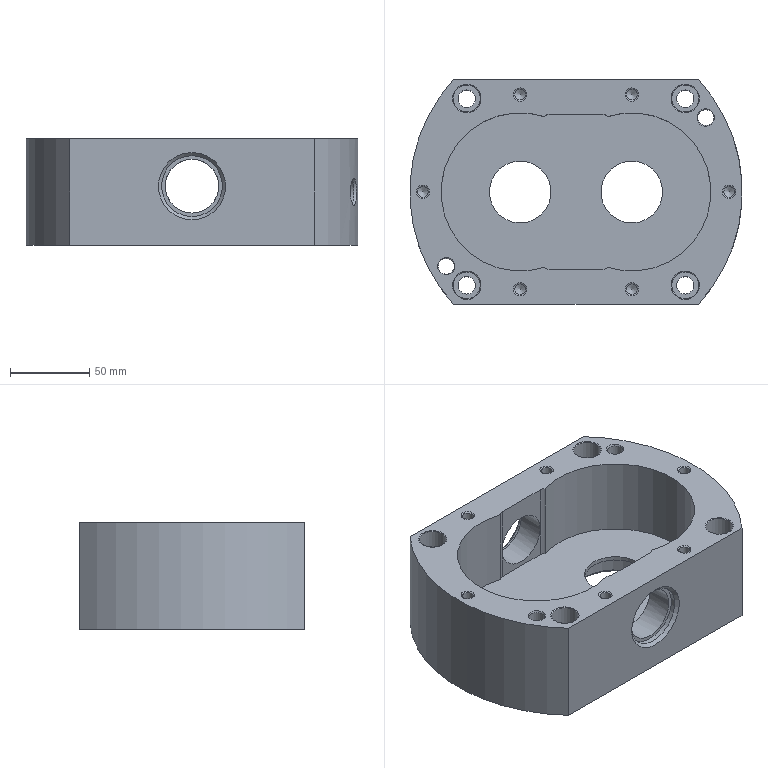NC program | NX | posted with a generic post | part box 210 x 142 x 67.4 mm
Lines 86 to 894 of 83330:
(HOLE_MILLING_COPY_COPY , TOOL : D10)
N146 T10 M6
N148 G54
N150 G17 G0 G90 X-35.25 Y0. B0. C0. S3000 M3
N152 G43 Z30. H10
N154 Z1.5
N156 G94 G3 X-36.5 Y1.25 R1.25 F2200.
N158 X-37.75 Y0. R1.25
N160 X-37.75 Y0. Z1.28 I2.5 J0.
N162 X-37.75 Y0. Z1.06 I2.5 J0.
N164 X-37.75 Y0. Z0.84 I2.5 J0.
N166 X-37.75 Y0. Z0.62 I2.5 J0.
N168 X-37.75 Y0. Z0.4 I2.5 J0.
N170 X-37.75 Y0. Z0.18 I2.5 J0.
N172 X-37.75 Y0. Z-0.04 I2.5 J0.
N174 X-37.75 Y0. Z-0.26 I2.5 J0.
N176 X-37.75 Y0. Z-0.48 I2.5 J0.
N178 X-37.75 Y0. Z-0.7 I2.5 J0.
N180 X-37.75 Y0. Z-0.92 I2.5 J0.
N182 X-37.75 Y0. Z-1.14 I2.5 J0.
N184 X-37.75 Y0. Z-1.36 I2.5 J0.
N186 X-37.75 Y0. Z-1.58 I2.5 J0.
N188 X-37.75 Y0. Z-1.8 I2.5 J0.
N190 X-37.75 Y0. Z-2.02 I2.5 J0.
N192 X-37.75 Y0. Z-2.24 I2.5 J0.
N194 X-37.75 Y0. Z-2.46 I2.5 J0.
N196 X-37.75 Y0. Z-2.68 I2.5 J0.
N198 X-37.75 Y0. Z-2.9 I2.5 J0.
N200 X-37.75 Y0. Z-3.12 I2.5 J0.
N202 X-37.75 Y0. Z-3.34 I2.5 J0.
N204 X-37.75 Y0. Z-3.56 I2.5 J0.
N206 X-37.75 Y0. Z-3.78 I2.5 J0.
N208 X-37.75 Y0. Z-4. I2.5 J0.
N210 X-37.75 Y0. Z-4.22 I2.5 J0.
N212 X-37.75 Y0. Z-4.44 I2.5 J0.
N214 X-37.75 Y0. Z-4.66 I2.5 J0.
N216 X-37.75 Y0. Z-4.88 I2.5 J0.
N218 X-37.75 Y0. Z-5.1 I2.5 J0.
N220 X-37.75 Y0. Z-5.32 I2.5 J0.
N222 X-37.75 Y0. Z-5.54 I2.5 J0.
N224 X-37.75 Y0. Z-5.76 I2.5 J0.
N226 X-37.75 Y0. Z-5.98 I2.5 J0.
N228 X-37.75 Y0. Z-6.2 I2.5 J0.
N230 X-37.75 Y0. Z-6.42 I2.5 J0.
N232 X-37.75 Y0. Z-6.64 I2.5 J0.
N234 X-37.75 Y0. Z-6.86 I2.5 J0.
N236 X-37.75 Y0. Z-7.08 I2.5 J0.
N238 X-37.75 Y0. Z-7.3 I2.5 J0.
N240 X-37.75 Y0. Z-7.52 I2.5 J0.
N242 X-37.75 Y0. Z-7.74 I2.5 J0.
N244 X-37.75 Y0. Z-7.96 I2.5 J0.
N246 X-37.75 Y0. Z-8.18 I2.5 J0.
N248 X-37.75 Y0. Z-8.4 I2.5 J0.
N250 X-37.75 Y0. Z-8.62 I2.5 J0.
N252 X-37.75 Y0. Z-8.84 I2.5 J0.
N254 X-37.75 Y0. Z-9.06 I2.5 J0.
N256 X-37.75 Y0. Z-9.28 I2.5 J0.
N258 X-37.75 Y0. Z-9.5 I2.5 J0.
N260 X-37.75 Y0. Z-9.72 I2.5 J0.
N262 X-37.75 Y0. Z-9.94 I2.5 J0.
N264 X-37.75 Y0. Z-10.16 I2.5 J0.
N266 X-37.75 Y0. Z-10.38 I2.5 J0.
N268 X-37.75 Y0. Z-10.6 I2.5 J0.
N270 X-37.75 Y0. Z-10.82 I2.5 J0.
N272 X-37.75 Y0. Z-11.04 I2.5 J0.
N274 X-37.75 Y0. Z-11.26 I2.5 J0.
N276 X-37.75 Y0. Z-11.48 I2.5 J0.
N278 X-37.75 Y0. Z-11.7 I2.5 J0.
N280 X-37.75 Y0. Z-11.92 I2.5 J0.
N282 X-37.75 Y0. Z-12.14 I2.5 J0.
N284 X-37.75 Y0. Z-12.36 I2.5 J0.
N286 X-37.75 Y0. Z-12.58 I2.5 J0.
N288 X-37.75 Y0. Z-12.8 I2.5 J0.
N290 X-37.75 Y0. Z-13.02 I2.5 J0.
N292 X-37.75 Y0. Z-13.24 I2.5 J0.
N294 X-37.75 Y0. Z-13.46 I2.5 J0.
N296 X-37.75 Y0. Z-13.68 I2.5 J0.
N298 X-37.75 Y0. Z-13.9 I2.5 J0.
N300 X-37.75 Y0. Z-14.12 I2.5 J0.
N302 X-37.75 Y0. Z-14.34 I2.5 J0.
N304 X-37.75 Y0. Z-14.56 I2.5 J0.
N306 X-33.613 Y1.889 Z-14.7 R-2.5
N308 X-37.181 Y1.641 R2.534
N310 X-36.968 Y-1.952 R2.566
N312 X-33.277 Y-1.768 R2.618
N314 X-33.451 Y2.013 R2.681
N316 X-37.284 Y1.85 R2.717
N318 X-37.132 Y-2.073 R2.781
N320 X-33.157 Y-1.933 R2.817
N322 X-33.285 Y2.131 R2.881
N324 X-37.401 Y2.017 R2.917
N326 X-37.3 Y-2.189 R2.98
N328 X-33.042 Y-2.102 R3.017
N330 X-33.115 Y2.246 R3.08
N332 X-37.514 Y2.188 R3.116
N334 X-37.472 Y-2.301 R3.18
N336 X-32.932 Y-2.275 R3.216
N338 X-32.941 Y2.355 R3.28
N340 X-37.622 Y2.363 R3.316
N342 X-37.648 Y-2.408 R3.38
N344 X-32.826 Y-2.452 R3.416
N346 X-32.763 Y2.459 R3.479
N348 X-37.725 Y2.541 R3.516
N350 X-37.827 Y-2.51 R3.579
N352 X-32.726 Y-2.632 R3.615
N354 X-32.581 Y2.559 R3.679
N356 X-37.823 Y2.724 R3.715
N358 X-38.011 Y-2.607 R3.779
N360 X-32.63 Y-2.816 R3.815
N362 X-32.396 Y2.653 R3.878
N364 X-37.916 Y2.91 R3.915
N366 X-38.198 Y-2.699 R3.978
N368 X-32.539 Y-3.004 R4.014
N370 X-32.208 Y2.743 R4.078
N372 X-38.004 Y3.099 R4.114
N374 X-38.388 Y-2.785 R4.178
N376 X-32.454 Y-3.195 R4.214
N378 X-32.015 Y2.827 R4.277
N380 X-38.086 Y3.292 R4.314
N382 X-38.582 Y-2.867 R4.377
N384 X-32.374 Y-3.39 R4.413
N386 X-31.82 Y2.905 R4.477
N388 X-38.164 Y3.488 R4.513
N390 X-38.779 Y-2.943 R4.577
N392 X-32.3 Y-3.587 R4.613
N394 X-31.622 Y2.979 R4.676
N396 X-38.236 Y3.687 R4.713
N398 X-38.979 Y-3.014 R4.776
N400 X-32.23 Y-3.788 R4.812
N402 X-31.42 Y3.047 R4.876
N404 X-38.302 Y3.889 R4.912
N406 X-39.182 Y-3.079 R4.976
N408 X-32.167 Y-3.991 R5.012
N410 X-31.215 Y3.109 R5.075
N412 X-38.363 Y4.094 R5.112
N414 X-39.388 Y-3.138 R5.175
N416 X-32.108 Y-4.198 R5.211
N418 X-31.008 Y3.166 R5.275
N420 X-38.418 Y4.302 R5.311
N422 X-39.596 Y-3.192 R5.375
N424 X-32.056 Y-4.407 R5.411
N426 X-30.798 Y3.217 R5.474
N428 X-38.468 Y4.513 R5.511
N430 X-39.808 Y-3.241 R5.574
N432 X-32.009 Y-4.619 R5.61
N434 X-30.586 Y3.263 R5.674
N436 X-38.512 Y4.725 R5.71
N438 X-40.021 Y-3.283 R5.774
N440 X-31.968 Y-4.833 R5.81
N442 X-30.371 Y3.302 R5.873
N444 X-38.55 Y4.941 R5.91
N446 X-40.238 Y-3.32 R5.973
N448 X-31.933 Y-5.049 R6.009
N450 X-30.154 Y3.336 R6.073
N452 X-38.582 Y5.158 R6.109
N454 X-40.456 Y-3.351 R6.173
N456 X-31.904 Y-5.268 R6.209
N458 X-29.934 Y3.364 R6.272
N460 X-38.608 Y5.378 R6.309
N462 X-40.676 Y-3.376 R6.372
N464 X-31.881 Y-5.489 R6.408
N466 X-29.713 Y3.386 R6.472
N468 X-38.629 Y5.6 R6.508
N470 X-40.899 Y-3.394 R6.572
N472 X-31.864 Y-5.711 R6.608
N474 X-29.49 Y3.401 R6.672
N476 X-38.643 Y5.823 R6.708
N478 X-41.123 Y-3.407 R6.771
N480 X-31.853 Y-5.936 R6.808
N482 X-29.265 Y3.411 R6.871
N484 X-38.651 Y6.049 R6.907
N486 X-41.349 Y-3.414 R6.971
N488 X-31.848 Y-6.162 R7.007
N490 X-29.038 Y3.415 R7.071
N492 X-38.653 Y6.275 R7.107
N494 X-41.576 Y-3.414 R7.17
N496 X-31.849 Y-6.389 R7.207
N498 X-28.81 Y3.412 R7.27
N500 X-38.648 Y6.504 R7.306
N502 X-41.805 Y-3.408 R7.37
N504 X-31.856 Y-6.618 R7.406
N506 X-28.58 Y3.403 R7.47
N508 X-38.638 Y6.733 R7.506
N510 X-42.035 Y-3.396 R7.569
N512 X-31.87 Y-6.849 R7.606
N514 X-28.35 Y3.388 R7.669
N516 X-38.621 Y6.964 R7.705
N518 X-42.266 Y-3.378 R7.769
N520 X-31.89 Y-7.08 R7.805
N522 X-28.118 Y3.366 R7.869
N524 X-38.598 Y7.196 R7.905
N526 X-42.498 Y-3.353 R7.968
N528 X-31.916 Y-7.312 R8.005
N530 X-27.885 Y3.339 R8.068
N532 X-38.568 Y7.429 R8.104
N534 X-42.732 Y-3.322 R8.168
N536 X-31.949 Y-7.545 R8.204
N538 X-27.652 Y3.304 R8.268
N540 X-38.532 Y7.662 R8.304
N542 X-42.965 Y-3.285 R8.367
N544 X-31.988 Y-7.779 R8.404
N546 X-27.417 Y3.264 R8.467
N548 X-38.49 Y7.896 R8.503
N550 X-43.2 Y-3.241 R8.567
N552 X-32.034 Y-8.014 R8.603
N554 X-27.183 Y3.217 R8.667
N556 X-38.441 Y8.131 R8.703
N558 X-43.435 Y-3.191 R8.766
N560 X-32.086 Y-8.248 R8.803
N562 X-26.948 Y3.163 R8.866
N564 X-38.386 Y8.366 R8.902
N566 X-43.67 Y-3.134 R8.966
N568 X-32.144 Y-8.483 R9.002
N570 X-26.713 Y3.103 R9.066
N572 X-38.324 Y8.601 R9.102
N574 X-43.905 Y-3.07 R9.165
N576 X-32.209 Y-8.718 R9.202
N578 X-26.477 Y3.036 R9.265
N580 X-38.256 Y8.836 R9.301
N582 X-44.14 Y-3.001 R9.365
N584 X-32.281 Y-8.953 R9.401
N586 X-26.242 Y2.963 R9.465
N588 X-38.181 Y9.071 R9.501
N590 X-44.376 Y-2.924 R9.564
N592 X-32.359 Y-9.188 R9.601
N594 X-26.007 Y2.884 R9.664
N596 X-38.1 Y9.306 R9.7
N598 X-44.61 Y-2.841 R9.764
N600 X-32.444 Y-9.423 R9.8
N602 X-25.772 Y2.797 R9.864
N604 X-38.012 Y9.54 R9.9
N606 X-44.845 Y-2.752 R9.963
N608 X-32.535 Y-9.657 R10.
N610 X-25.538 Y2.705 R10.063
N612 X-37.917 Y9.774 R10.099
N614 X-45.079 Y-2.656 R10.163
N616 X-32.632 Y-9.89 R10.199
N618 X-25.305 Y2.605 R10.263
N620 X-37.816 Y10.007 R10.299
N622 X-45.312 Y-2.553 R10.362
N624 X-32.737 Y-10.123 R10.399
N626 X-25.072 Y2.499 R10.462
N628 X-37.709 Y10.239 R10.498
N630 X-45.544 Y-2.444 R10.562
N632 X-32.848 Y-10.355 R10.598
N634 X-24.84 Y2.387 R10.662
N636 X-37.595 Y10.47 R10.698
N638 X-45.775 Y-2.328 R10.761
N640 X-32.965 Y-10.586 R10.798
N642 X-24.61 Y2.268 R10.861
N644 X-37.474 Y10.701 R10.897
N646 X-46.005 Y-2.206 R10.961
N648 X-33.089 Y-10.815 R10.997
N650 X-24.38 Y2.142 R11.061
N652 X-37.347 Y10.929 R11.097
N654 X-46.234 Y-2.077 R11.161
N656 X-33.219 Y-11.043 R11.197
N658 X-24.152 Y2.01 R11.26
N660 X-37.213 Y11.157 R11.297
N662 X-46.461 Y-1.942 R11.36
N664 X-33.356 Y-11.27 R11.396
N666 X-23.926 Y1.872 R11.46
N668 X-37.073 Y11.383 R11.496
N670 X-46.687 Y-1.8 R11.56
N672 X-33.5 Y-11.495 R11.596
N674 X-23.701 Y1.727 R11.659
N676 X-36.926 Y11.607 R11.696
N678 X-46.911 Y-1.652 R11.759
N680 X-33.65 Y-11.718 R11.795
N682 X-23.478 Y1.575 R11.859
N684 X-36.773 Y11.829 R11.895
N686 X-47.133 Y-1.497 R11.959
N688 X-33.806 Y-11.94 R11.995
N690 X-23.257 Y1.417 R12.058
N692 X-36.613 Y12.049 R12.095
N694 X-47.353 Y-1.335 R12.158
N696 X-33.969 Y-12.159 R12.194
N698 X-23.038 Y1.252 R12.258
N700 X-36.447 Y12.268 R12.294
N702 X-47.571 Y-1.168 R12.358
N704 X-34.139 Y-12.376 R12.394
N706 X-22.821 Y1.082 R12.457
N708 X-36.274 Y12.483 R12.494
N710 X-47.786 Y-0.994 R12.557
N712 X-34.314 Y-12.59 R12.593
N714 X-22.607 Y0.904 R12.657
N716 X-36.095 Y12.697 R12.693
N718 X-47.999 Y-0.813 R12.757
N720 X-34.496 Y-12.802 R12.793
N722 X-22.396 Y0.721 R12.856
N724 X-35.91 Y12.907 R12.893
N726 X-48.209 Y-0.626 R12.956
N728 X-34.685 Y-13.012 R12.992
N730 X-22.187 Y0.531 R13.056
N732 X-35.719 Y13.116 R13.092
N734 X-48.417 Y-0.433 R13.156
N736 X-34.879 Y-13.218 R13.192
N738 X-21.981 Y0.334 R13.255
N740 X-35.521 Y13.321 R13.292
N742 X-48.621 Y-0.234 R13.355
N744 X-35.08 Y-13.422 R13.391
N746 X-21.778 Y0.132 R13.455
N748 X-35.317 Y13.523 R13.491
N750 X-48.823 Y-0.029 R13.555
N752 X-35.287 Y-13.623 R13.591
N754 X-21.578 Y-0.077 R13.654
N756 X-35.107 Y13.722 R13.691
N758 X-49.021 Y0.183 R13.754
N760 X-35.501 Y-13.82 R13.79
N762 X-21.381 Y-0.291 R13.854
N764 X-34.89 Y13.917 R13.89
N766 X-49.216 Y0.401 R13.954
N768 X-35.72 Y-14.014 R13.99
N770 X-21.188 Y-0.512 R14.053
N772 X-34.668 Y14.109 R14.09
N774 X-49.408 Y0.625 R14.153
N776 X-35.945 Y-14.204 R14.189
N778 X-20.998 Y-0.739 R14.253
N780 X-34.44 Y14.298 R14.289
N782 X-49.595 Y0.855 R14.353
N784 X-36.177 Y-14.391 R14.389
N786 X-20.812 Y-0.972 R14.452
N788 X-34.206 Y14.483 R14.489
N790 X-49.779 Y1.09 R14.552
N792 X-36.414 Y-14.574 R14.588
N794 X-20.63 Y-1.21 R14.652
N796 X-33.966 Y14.664 R14.688
N798 X-49.96 Y1.332 R14.752
N800 X-36.657 Y-14.753 R14.788
N802 X-20.452 Y-1.455 R14.851
N804 X-33.72 Y14.841 R14.888
N806 X-50.136 Y1.579 R14.951
N808 X-36.906 Y-14.928 R14.987
N810 X-20.278 Y-1.705 R15.051
N812 X-33.468 Y15.014 R15.087
N814 X-50.308 Y1.832 R15.151
N816 X-37.16 Y-15.098 R15.187
N818 X-20.108 Y-1.961 R15.25
N820 X-33.21 Y15.182 R15.287
N822 X-50.475 Y2.091 R15.35
N824 X-37.42 Y-15.265 R15.386
N826 X-19.942 Y-2.223 R15.45
N828 X-32.948 Y15.346 R15.486
N830 X-50.639 Y2.356 R15.55
N832 X-37.686 Y-15.427 R15.586
N834 X-19.781 Y-2.49 R15.649
N836 X-32.679 Y15.506 R15.686
N838 X-50.797 Y2.626 R15.749
N840 X-37.957 Y-15.584 R15.785
N842 X-19.625 Y-2.763 R15.849
N844 X-32.405 Y15.661 R15.885
N846 X-50.951 Y2.901 R15.949
N848 X-38.234 Y-15.736 R15.985
N850 X-19.474 Y-3.041 R16.049
N852 X-32.126 Y15.811 R16.085
N854 X-51.1 Y3.182 R16.148
N856 X-38.516 Y-15.884 R16.185
N858 X-19.327 Y-3.324 R16.248
N860 X-31.841 Y15.956 R16.284
N862 X-51.244 Y3.468 R16.348
N864 X-38.803 Y-16.027 R16.384
N866 X-19.186 Y-3.613 R16.448
N868 X-31.551 Y16.096 R16.484
N870 X-51.383 Y3.759 R16.547
N872 X-39.096 Y-16.164 R16.584
N874 X-19.049 Y-3.906 R16.647
N876 X-31.256 Y16.231 R16.683
N878 X-51.517 Y4.055 R16.747
N880 X-39.393 Y-16.296 R16.783
N882 X-18.918 Y-4.205 R16.847
N884 X-30.956 Y16.361 R16.883
N886 X-51.646 Y4.356 R16.946
N888 X-39.696 Y-16.423 R16.983
N890 X-18.792 Y-4.509 R17.046
N892 X-30.651 Y16.485 R17.082
N894 X-51.769 Y4.662 R17.146
N896 X-40.003 Y-16.545 R17.182
N898 X-18.672 Y-4.817 R17.246
N900 X-30.342 Y16.603 R17.282
N902 X-51.886 Y4.973 R17.345
N904 X-40.315 Y-16.66 R17.382
N906 X-18.557 Y-5.131 R17.445
N908 X-30.027 Y16.716 R17.481
N910 X-51.998 Y5.289 R17.545
N912 X-40.632 Y-16.771 R17.581
N914 X-18.449 Y-5.449 R17.645
N916 X-29.708 Y16.823 R17.681
N918 X-52.104 Y5.609 R17.744
N920 X-40.953 Y-16.875 R17.781
N922 X-18.346 Y-5.771 R17.844
N924 X-29.385 Y16.925 R17.88
N926 X-52.203 Y5.934 R17.944
N928 X-41.279 Y-16.973 R17.98
N930 X-18.249 Y-6.098 R18.044
N932 X-29.057 Y17.02 R18.08
N934 X-52.297 Y6.263 R18.143
N936 X-41.609 Y-17.065 R18.18
N938 X-18.158 Y-6.43 R18.243
N940 X-28.724 Y17.109 R18.279
N942 X-52.385 Y6.597 R18.343
N944 X-41.943 Y-17.151 R18.379
N946 X-18.073 Y-6.765 R18.443
N948 X-28.388 Y17.192 R18.479
N950 X-52.466 Y6.934 R18.542
N952 X-42.282 Y-17.231 R18.579
N954 X-17.995 Y-7.105 R18.642
N956 X-28.047 Y17.268 R18.678
N958 X-52.542 Y7.276 R18.742
N960 X-42.625 Y-17.304 R18.778
N962 X-17.923 Y-7.448 R18.842
N964 X-27.703 Y17.338 R18.878
N966 X-52.61 Y7.622 R18.941
N968 X-42.971 Y-17.371 R18.978
N970 X-17.858 Y-7.796 R19.041
N972 X-27.354 Y17.402 R19.077
N974 X-52.672 Y7.971 R19.141
N976 X-43.321 Y-17.431 R19.177
N978 X-17.799 Y-8.147 R19.241
N980 X-27.002 Y17.458 R19.277
N982 X-52.727 Y8.324 R19.34
N984 X-43.675 Y-17.484 R19.377
N986 X-17.747 Y-8.502 R19.44
N988 X-26.646 Y17.508 R19.476
N990 X-52.776 Y8.681 R19.54
N992 X-44.033 Y-17.531 R19.576
N994 X-17.702 Y-8.861 R19.64
N996 X-26.287 Y17.552 R19.676
N998 X-52.818 Y9.041 R19.739
N1000 X-44.394 Y-17.571 R19.776
N1002 X-17.664 Y-9.222 R19.839
N1004 X-25.925 Y17.588 R19.875
N1006 X-52.852 Y9.405 R19.939
N1008 X-44.758 Y-17.603 R19.975
N1010 X-17.633 Y-9.588 R20.039
N1012 X-25.559 Y17.617 R20.075
N1014 X-52.88 Y9.771 R20.138
N1016 X-45.125 Y-17.629 R20.175
N1018 X-17.609 Y-9.956 R20.238
N1020 X-25.19 Y17.639 R20.274
N1022 X-52.9 Y10.141 R20.338
N1024 X-45.496 Y-17.647 R20.374
N1026 X-17.592 Y-10.327 R20.438
N1028 X-24.818 Y17.654 R20.474
N1030 X-52.913 Y10.514 R20.537
N1032 X-45.869 Y-17.659 R20.574
N1034 X-17.583 Y-10.701 R20.637
N1036 X-24.443 Y17.661 R20.673
N1038 X-52.919 Y10.889 R20.737
N1040 X-46.245 Y-17.662 R20.773
N1042 X-17.581 Y-11.078 R20.837
N1044 X-24.066 Y17.662 R20.873
N1046 X-52.918 Y11.267 R20.937
N1048 X-46.624 Y-17.659 R20.973
N1050 X-17.586 Y-11.457 R21.036
N1052 X-23.686 Y17.654 R21.073
N1054 X-52.909 Y11.648 R21.136
N1056 X-47.005 Y-17.648 R21.172
N1058 X-17.599 Y-11.839 R21.236
N1060 X-23.304 Y17.639 R21.272
N1062 X-52.892 Y12.031 R21.336
N1064 X-47.388 Y-17.629 R21.372
N1066 X-17.619 Y-12.223 R21.435
N1068 X-22.919 Y17.617 R21.472
N1070 X-52.868 Y12.416 R21.535
N1072 X-47.774 Y-17.603 R21.571
N1074 X-17.647 Y-12.609 R21.635
N1076 X-22.533 Y17.587 R21.671
N1078 X-52.836 Y12.803 R21.735
N1080 X-48.161 Y-17.568 R21.771
N1082 X-17.683 Y-12.998 R21.834
N1084 X-22.144 Y17.549 R21.871
N1086 X-52.796 Y13.192 R21.934
N1088 X-48.551 Y-17.527 R21.97
N1090 X-17.727 Y-13.388 R22.034
N1092 X-21.754 Y17.503 R22.07
N1094 X-52.748 Y13.583 R22.134
N1096 X-48.942 Y-17.477 R22.17
N1098 X-17.778 Y-13.779 R22.233
N1100 X-21.362 Y17.449 R22.27
N1102 X-52.693 Y13.976 R22.333
N1104 X-49.335 Y-17.419 R22.369
N1106 X-17.838 Y-14.173 R22.433
N1108 X-20.968 Y17.387 R22.469
N1110 X-52.629 Y14.37 R22.533
N1112 X-49.729 Y-17.353 R22.569
N1114 X-17.906 Y-14.568 R22.632
N1116 X-20.573 Y17.318 R22.669
N1118 X-52.558 Y14.765 R22.732
N1120 X-50.099 Y-17.323 R22.784
N1122 X-17.981 Y-14.964 R22.816
N1124 X-20.286 Y17.269 R22.85
N1126 X-17.981 Y-14.964 R-22.85
N1128 X-19.134 Y1.153 R11.425
N1130 X-35.25 Y0. R11.425
N1132 G0 Z30.
N1134 X35.25
N1136 Z1.5
N1138 G3 X34. Y1.25 R1.25
N1140 X32.75 Y0. R1.25
N1142 X32.75 Y0. Z1.28 I2.5 J0.
N1144 X32.75 Y0. Z1.06 I2.5 J0.
N1146 X32.75 Y0. Z0.84 I2.5 J0.
N1148 X32.75 Y0. Z0.62 I2.5 J0.
N1150 X32.75 Y0. Z0.4 I2.5 J0.
N1152 X32.75 Y0. Z0.18 I2.5 J0.
N1154 X32.75 Y0. Z-0.04 I2.5 J0.
N1156 X32.75 Y0. Z-0.26 I2.5 J0.
N1158 X32.75 Y0. Z-0.48 I2.5 J0.
N1160 X32.75 Y0. Z-0.7 I2.5 J0.
N1162 X32.75 Y0. Z-0.92 I2.5 J0.
N1164 X32.75 Y0. Z-1.14 I2.5 J0.
N1166 X32.75 Y0. Z-1.36 I2.5 J0.
N1168 X32.75 Y0. Z-1.58 I2.5 J0.
N1170 X32.75 Y0. Z-1.8 I2.5 J0.
N1172 X32.75 Y0. Z-2.02 I2.5 J0.
N1174 X32.75 Y0. Z-2.24 I2.5 J0.
N1176 X32.75 Y0. Z-2.46 I2.5 J0.
N1178 X32.75 Y0. Z-2.68 I2.5 J0.
N1180 X32.75 Y0. Z-2.9 I2.5 J0.
N1182 X32.75 Y0. Z-3.12 I2.5 J0.
N1184 X32.75 Y0. Z-3.34 I2.5 J0.
N1186 X32.75 Y0. Z-3.56 I2.5 J0.
N1188 X32.75 Y0. Z-3.78 I2.5 J0.
N1190 X32.75 Y0. Z-4. I2.5 J0.
N1192 X32.75 Y0. Z-4.22 I2.5 J0.
N1194 X32.75 Y0. Z-4.44 I2.5 J0.
N1196 X32.75 Y0. Z-4.66 I2.5 J0.
N1198 X32.75 Y0. Z-4.88 I2.5 J0.
N1200 X32.75 Y0. Z-5.1 I2.5 J0.
N1202 X32.75 Y0. Z-5.32 I2.5 J0.
N1204 X32.75 Y0. Z-5.54 I2.5 J0.
N1206 X32.75 Y0. Z-5.76 I2.5 J0.
N1208 X32.75 Y0. Z-5.98 I2.5 J0.
N1210 X32.75 Y0. Z-6.2 I2.5 J0.
N1212 X32.75 Y0. Z-6.42 I2.5 J0.
N1214 X32.75 Y0. Z-6.64 I2.5 J0.
N1216 X32.75 Y0. Z-6.86 I2.5 J0.
N1218 X32.75 Y0. Z-7.08 I2.5 J0.
N1220 X32.75 Y0. Z-7.3 I2.5 J0.
N1222 X32.75 Y0. Z-7.52 I2.5 J0.
N1224 X32.75 Y0. Z-7.74 I2.5 J0.
N1226 X32.75 Y0. Z-7.96 I2.5 J0.
N1228 X32.75 Y0. Z-8.18 I2.5 J0.
N1230 X32.75 Y0. Z-8.4 I2.5 J0.
N1232 X32.75 Y0. Z-8.62 I2.5 J0.
N1234 X32.75 Y0. Z-8.84 I2.5 J0.
N1236 X32.75 Y0. Z-9.06 I2.5 J0.
N1238 X32.75 Y0. Z-9.28 I2.5 J0.
N1240 X32.75 Y0. Z-9.5 I2.5 J0.
N1242 X32.75 Y0. Z-9.72 I2.5 J0.
N1244 X32.75 Y0. Z-9.94 I2.5 J0.
N1246 X32.75 Y0. Z-10.16 I2.5 J0.
N1248 X32.75 Y0. Z-10.38 I2.5 J0.
N1250 X32.75 Y0. Z-10.6 I2.5 J0.
N1252 X32.75 Y0. Z-10.82 I2.5 J0.
N1254 X32.75 Y0. Z-11.04 I2.5 J0.
N1256 X32.75 Y0. Z-11.26 I2.5 J0.
N1258 X32.75 Y0. Z-11.48 I2.5 J0.
N1260 X32.75 Y0. Z-11.7 I2.5 J0.
N1262 X32.75 Y0. Z-11.92 I2.5 J0.
N1264 X32.75 Y0. Z-12.14 I2.5 J0.
N1266 X32.75 Y0. Z-12.36 I2.5 J0.
N1268 X32.75 Y0. Z-12.58 I2.5 J0.
N1270 X32.75 Y0. Z-12.8 I2.5 J0.
N1272 X32.75 Y0. Z-13.02 I2.5 J0.
N1274 X32.75 Y0. Z-13.24 I2.5 J0.
N1276 X32.75 Y0. Z-13.46 I2.5 J0.
N1278 X32.75 Y0. Z-13.68 I2.5 J0.
N1280 X32.75 Y0. Z-13.9 I2.5 J0.
N1282 X32.75 Y0. Z-14.12 I2.5 J0.
N1284 X32.75 Y0. Z-14.34 I2.5 J0.
N1286 X32.75 Y0. Z-14.56 I2.5 J0.
N1288 X36.887 Y1.889 Z-14.7 R-2.5
N1290 X33.319 Y1.641 R2.534
N1292 X33.532 Y-1.952 R2.566
N1294 X37.223 Y-1.768 R2.618
N1296 X37.049 Y2.013 R2.681
N1298 X33.216 Y1.85 R2.717
N1300 X33.368 Y-2.073 R2.781
N1302 X37.343 Y-1.933 R2.817
N1304 X37.215 Y2.131 R2.881
N1306 X33.099 Y2.017 R2.917
N1308 X33.2 Y-2.189 R2.98
N1310 X37.458 Y-2.102 R3.017
N1312 X37.385 Y2.246 R3.08
N1314 X32.986 Y2.188 R3.116
N1316 X33.028 Y-2.301 R3.18
N1318 X37.568 Y-2.275 R3.216
N1320 X37.559 Y2.355 R3.28
N1322 X32.878 Y2.363 R3.316
N1324 X32.852 Y-2.408 R3.38
N1326 X37.674 Y-2.452 R3.416
N1328 X37.737 Y2.459 R3.479
N1330 X32.775 Y2.541 R3.516
N1332 X32.673 Y-2.51 R3.579
N1334 X37.774 Y-2.632 R3.615
N1336 X37.919 Y2.559 R3.679
N1338 X32.677 Y2.724 R3.715
N1340 X32.489 Y-2.607 R3.779
N1342 X37.87 Y-2.816 R3.815
N1344 X38.104 Y2.653 R3.878
N1346 X32.584 Y2.91 R3.915
N1348 X32.302 Y-2.699 R3.978
N1350 X37.961 Y-3.004 R4.014
N1352 X38.292 Y2.743 R4.078
N1354 X32.496 Y3.099 R4.114
N1356 X32.112 Y-2.785 R4.178
N1358 X38.046 Y-3.195 R4.214
N1360 X38.485 Y2.827 R4.277
N1362 X32.414 Y3.292 R4.314
N1364 X31.918 Y-2.867 R4.377
N1366 X38.126 Y-3.39 R4.413
N1368 X38.68 Y2.905 R4.477
N1370 X32.336 Y3.488 R4.513
N1372 X31.721 Y-2.943 R4.577
N1374 X38.2 Y-3.587 R4.613
N1376 X38.878 Y2.979 R4.676
N1378 X32.264 Y3.687 R4.713
N1380 X31.521 Y-3.014 R4.776
N1382 X38.27 Y-3.788 R4.812
N1384 X39.08 Y3.047 R4.876
N1386 X32.198 Y3.889 R4.912
N1388 X31.318 Y-3.079 R4.976
N1390 X38.333 Y-3.991 R5.012
N1392 X39.285 Y3.109 R5.075
N1394 X32.137 Y4.094 R5.112
N1396 X31.112 Y-3.138 R5.175
N1398 X38.392 Y-4.198 R5.211
N1400 X39.492 Y3.166 R5.275
N1402 X32.082 Y4.302 R5.311
N1404 X30.904 Y-3.192 R5.375
N1406 X38.444 Y-4.407 R5.411
N1408 X39.702 Y3.217 R5.474
N1410 X32.032 Y4.513 R5.511
N1412 X30.692 Y-3.241 R5.574
N1414 X38.491 Y-4.619 R5.61
N1416 X39.914 Y3.263 R5.674
N1418 X31.988 Y4.725 R5.71
N1420 X30.479 Y-3.283 R5.774
N1422 X38.532 Y-4.833 R5.81
N1424 X40.129 Y3.302 R5.873
N1426 X31.95 Y4.941 R5.91
N1428 X30.262 Y-3.32 R5.973
N1430 X38.567 Y-5.049 R6.009
N1432 X40.346 Y3.336 R6.073
N1434 X31.918 Y5.158 R6.109
N1436 X30.044 Y-3.351 R6.173
N1438 X38.596 Y-5.268 R6.209
N1440 X40.566 Y3.364 R6.272
N1442 X31.892 Y5.378 R6.309
N1444 X29.824 Y-3.376 R6.372
N1446 X38.619 Y-5.489 R6.408
N1448 X40.787 Y3.386 R6.472
N1450 X31.871 Y5.6 R6.508
N1452 X29.601 Y-3.394 R6.572
N1454 X38.636 Y-5.711 R6.608
N1456 X41.01 Y3.401 R6.672
N1458 X31.857 Y5.823 R6.708
N1460 X29.377 Y-3.407 R6.771
N1462 X38.647 Y-5.936 R6.808
N1464 X41.235 Y3.411 R6.871
N1466 X31.849 Y6.049 R6.907
N1468 X29.151 Y-3.414 R6.971
N1470 X38.652 Y-6.162 R7.007
N1472 X41.462 Y3.415 R7.071
N1474 X31.847 Y6.275 R7.107
N1476 X28.924 Y-3.414 R7.17
N1478 X38.651 Y-6.389 R7.207
N1480 X41.69 Y3.412 R7.27
N1482 X31.852 Y6.504 R7.306
N1484 X28.695 Y-3.408 R7.37
N1486 X38.644 Y-6.618 R7.406
N1488 X41.92 Y3.403 R7.47
N1490 X31.862 Y6.733 R7.506
N1492 X28.465 Y-3.396 R7.569
N1494 X38.63 Y-6.849 R7.606
N1496 X42.15 Y3.388 R7.669
N1498 X31.879 Y6.964 R7.705
N1500 X28.234 Y-3.378 R7.769
N1502 X38.61 Y-7.08 R7.805
N1504 X42.382 Y3.366 R7.869
N1506 X31.902 Y7.196 R7.905
N1508 X28.002 Y-3.353 R7.968
N1510 X38.584 Y-7.312 R8.005
N1512 X42.615 Y3.339 R8.068
N1514 X31.932 Y7.429 R8.104
N1516 X27.768 Y-3.322 R8.168
N1518 X38.551 Y-7.545 R8.204
N1520 X42.848 Y3.304 R8.268
N1522 X31.968 Y7.662 R8.304
N1524 X27.535 Y-3.285 R8.367
N1526 X38.512 Y-7.779 R8.404
N1528 X43.083 Y3.264 R8.467
N1530 X32.01 Y7.896 R8.503
N1532 X27.3 Y-3.241 R8.567
N1534 X38.466 Y-8.014 R8.603
N1536 X43.317 Y3.217 R8.667
N1538 X32.059 Y8.131 R8.703
N1540 X27.065 Y-3.191 R8.766
N1542 X38.414 Y-8.248 R8.803
N1544 X43.552 Y3.163 R8.866
N1546 X32.114 Y8.366 R8.902
N1548 X26.83 Y-3.134 R8.966
N1550 X38.356 Y-8.483 R9.002
N1552 X43.787 Y3.103 R9.066
N1554 X32.176 Y8.601 R9.102
N1556 X26.595 Y-3.07 R9.165
N1558 X38.291 Y-8.718 R9.202
N1560 X44.023 Y3.036 R9.265
N1562 X32.244 Y8.836 R9.301
N1564 X26.36 Y-3.001 R9.365
N1566 X38.219 Y-8.953 R9.401
N1568 X44.258 Y2.963 R9.465
N1570 X32.319 Y9.071 R9.501
N1572 X26.124 Y-2.924 R9.564
N1574 X38.141 Y-9.188 R9.601
N1576 X44.493 Y2.884 R9.664
N1578 X32.4 Y9.306 R9.7
N1580 X25.89 Y-2.841 R9.764
N1582 X38.056 Y-9.423 R9.8
N1584 X44.728 Y2.797 R9.864
N1586 X32.488 Y9.54 R9.9
N1588 X25.655 Y-2.752 R9.963
N1590 X37.965 Y-9.657 R10.
N1592 X44.962 Y2.705 R10.063
N1594 X32.583 Y9.774 R10.099
N1596 X25.421 Y-2.656 R10.163
N1598 X37.868 Y-9.89 R10.199
N1600 X45.195 Y2.605 R10.263
N1602 X32.684 Y10.007 R10.299
N1604 X25.188 Y-2.553 R10.362
N1606 X37.763 Y-10.123 R10.399
N1608 X45.428 Y2.499 R10.462
N1610 X32.791 Y10.239 R10.498
N1612 X24.956 Y-2.444 R10.562
N1614 X37.652 Y-10.355 R10.598
N1616 X45.66 Y2.387 R10.662
N1618 X32.905 Y10.47 R10.698
N1620 X24.725 Y-2.328 R10.761
N1622 X37.535 Y-10.586 R10.798
N1624 X45.89 Y2.268 R10.861
N1626 X33.026 Y10.701 R10.897
N1628 X24.495 Y-2.206 R10.961
N1630 X37.411 Y-10.815 R10.997
N1632 X46.12 Y2.142 R11.061
N1634 X33.153 Y10.929 R11.097
N1636 X24.266 Y-2.077 R11.161
N1638 X37.281 Y-11.043 R11.197
N1640 X46.348 Y2.01 R11.26
N1642 X33.287 Y11.157 R11.297
N1644 X24.039 Y-1.942 R11.36
N1646 X37.144 Y-11.27 R11.396
N1648 X46.574 Y1.872 R11.46
N1650 X33.427 Y11.383 R11.496
N1652 X23.813 Y-1.8 R11.56
N1654 X37. Y-11.495 R11.596
N1656 X46.799 Y1.727 R11.659
N1658 X33.574 Y11.607 R11.696
N1660 X23.589 Y-1.652 R11.759
N1662 X36.85 Y-11.718 R11.795
N1664 X47.022 Y1.575 R11.859
N1666 X33.727 Y11.829 R11.895
N1668 X23.367 Y-1.497 R11.959
N1670 X36.694 Y-11.94 R11.995
N1672 X47.243 Y1.417 R12.058
N1674 X33.887 Y12.049 R12.095
N1676 X23.147 Y-1.335 R12.158
N1678 X36.531 Y-12.159 R12.194
N1680 X47.462 Y1.252 R12.258
N1682 X34.053 Y12.268 R12.294
N1684 X22.929 Y-1.168 R12.358
N1686 X36.361 Y-12.376 R12.394
N1688 X47.679 Y1.082 R12.457
N1690 X34.226 Y12.483 R12.494
N1692 X22.714 Y-0.994 R12.557
N1694 X36.186 Y-12.59 R12.593
N1696 X47.893 Y0.904 R12.657
N1698 X34.405 Y12.697 R12.693
N1700 X22.501 Y-0.813 R12.757
N1702 X36.004 Y-12.802 R12.793
N1704 X48.104 Y0.721 R12.856
N1706 X34.59 Y12.907 R12.893
N1708 X22.291 Y-0.626 R12.956
N1710 X35.815 Y-13.012 R12.992
N1712 X48.313 Y0.531 R13.056
N1714 X34.781 Y13.116 R13.092
N1716 X22.083 Y-0.433 R13.156
N1718 X35.621 Y-13.218 R13.192
N1720 X48.519 Y0.334 R13.255
N1722 X34.979 Y13.321 R13.292
N1724 X21.879 Y-0.234 R13.355
N1726 X35.42 Y-13.422 R13.391
N1728 X48.722 Y0.132 R13.455
N1730 X35.183 Y13.523 R13.491
N1732 X21.677 Y-0.029 R13.555
N1734 X35.213 Y-13.623 R13.591
N1736 X48.922 Y-0.077 R13.654
N1738 X35.393 Y13.722 R13.691
N1740 X21.479 Y0.183 R13.754
N1742 X34.999 Y-13.82 R13.79
N1744 X49.119 Y-0.291 R13.854
N1746 X35.61 Y13.917 R13.89
N1748 X21.284 Y0.401 R13.954
N1750 X34.78 Y-14.014 R13.99
N1752 X49.312 Y-0.512 R14.053
N1754 X35.832 Y14.109 R14.09
N1756 X21.092 Y0.625 R14.153